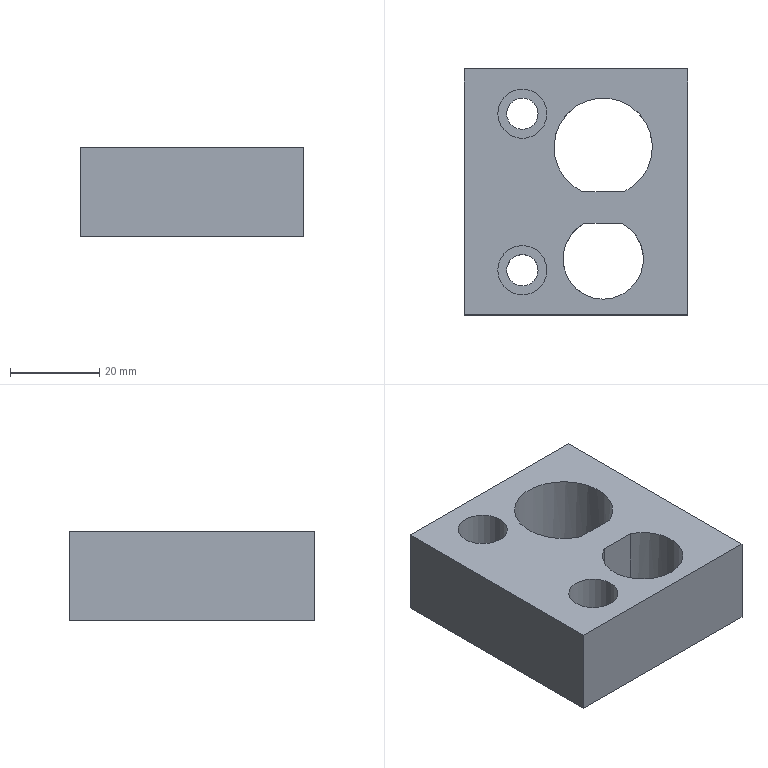Part | STEP file | lll_id706_x_t | 1 solid | 19 faces | box 50 x 55 x 20 mm | volume 39581 mm3 | plane 13 | cylinder 6 | commonest cylinder face diameters 7.009 x2 11.008 x2 18 x1 22 x1
STEP:
#1=CARTESIAN_POINT('',(395.083,115.522,-20.));
#2=VERTEX_POINT('',#1);
#3=CARTESIAN_POINT('',(395.083,107.06,-20.));
#4=VERTEX_POINT('',#3);
#5=CARTESIAN_POINT('',(395.083,100.,-20.));
#6=DIRECTION('',(0.,-1.,0.));
#7=VECTOR('',#6,1.);
#8=LINE('',#5,#7);
#9=EDGE_CURVE('',#2,#4,#8,.T.);
#10=ORIENTED_EDGE('',*,*,#9,.F.);
#11=CARTESIAN_POINT('',(383.917,115.522,-20.));
#12=VERTEX_POINT('',#11);
#13=CARTESIAN_POINT('',(389.5,125.,-20.));
#14=DIRECTION('',(0.,0.,1.));
#15=DIRECTION('',(1.,0.,0.));
#16=AXIS2_PLACEMENT_3D('',#13,#14,#15);
#17=CIRCLE('',#16,11.);
#18=EDGE_CURVE('',#2,#12,#17,.T.);
#19=ORIENTED_EDGE('',*,*,#18,.T.);
#20=CARTESIAN_POINT('',(383.917,107.06,-20.));
#21=VERTEX_POINT('',#20);
#22=CARTESIAN_POINT('',(383.917,100.,-20.));
#23=DIRECTION('',(0.,-1.,0.));
#24=VECTOR('',#23,1.);
#25=LINE('',#22,#24);
#26=EDGE_CURVE('',#12,#21,#25,.T.);
#27=ORIENTED_EDGE('',*,*,#26,.T.);
#28=CARTESIAN_POINT('',(389.5,100.,-20.));
#29=DIRECTION('',(0.,0.,-1.));
#30=DIRECTION('',(-1.,0.,0.));
#31=AXIS2_PLACEMENT_3D('',#28,#29,#30);
#32=CIRCLE('',#31,9.);
#33=EDGE_CURVE('',#4,#21,#32,.T.);
#34=ORIENTED_EDGE('',*,*,#33,.F.);
#35=EDGE_LOOP('',(#10,#19,#27,#34));
#36=FACE_BOUND('',#35,.T.);
#37=CARTESIAN_POINT('',(367.916,97.5,-20.));
#38=VERTEX_POINT('',#37);
#39=CARTESIAN_POINT('',(371.42,97.5,-20.));
#40=DIRECTION('',(0.,0.,-1.));
#41=DIRECTION('',(-1.,0.,0.));
#42=AXIS2_PLACEMENT_3D('',#39,#40,#41);
#43=CIRCLE('',#42,3.505);
#44=EDGE_CURVE('',#38,#38,#43,.T.);
#45=ORIENTED_EDGE('',*,*,#44,.F.);
#46=EDGE_LOOP('',(#45));
#47=FACE_BOUND('',#46,.T.);
#48=CARTESIAN_POINT('',(367.916,132.5,-20.));
#49=VERTEX_POINT('',#48);
#50=CARTESIAN_POINT('',(371.42,132.5,-20.));
#51=DIRECTION('',(0.,0.,-1.));
#52=DIRECTION('',(-1.,0.,0.));
#53=AXIS2_PLACEMENT_3D('',#50,#51,#52);
#54=CIRCLE('',#53,3.505);
#55=EDGE_CURVE('',#49,#49,#54,.T.);
#56=ORIENTED_EDGE('',*,*,#55,.F.);
#57=EDGE_LOOP('',(#56));
#58=FACE_BOUND('',#57,.T.);
#59=CARTESIAN_POINT('',(408.42,87.5,-20.));
#60=VERTEX_POINT('',#59);
#61=CARTESIAN_POINT('',(408.42,142.5,-20.));
#62=VERTEX_POINT('',#61);
#63=CARTESIAN_POINT('',(408.42,111.868,-20.));
#64=DIRECTION('',(0.,1.,0.));
#65=VECTOR('',#64,1.);
#66=LINE('',#63,#65);
#67=EDGE_CURVE('',#60,#62,#66,.T.);
#68=ORIENTED_EDGE('',*,*,#67,.F.);
#69=CARTESIAN_POINT('',(358.42,87.5,-20.));
#70=VERTEX_POINT('',#69);
#71=CARTESIAN_POINT('',(389.5,87.5,-20.));
#72=DIRECTION('',(1.,0.,0.));
#73=VECTOR('',#72,1.);
#74=LINE('',#71,#73);
#75=EDGE_CURVE('',#70,#60,#74,.T.);
#76=ORIENTED_EDGE('',*,*,#75,.F.);
#77=CARTESIAN_POINT('',(358.42,142.5,-20.));
#78=VERTEX_POINT('',#77);
#79=CARTESIAN_POINT('',(358.42,100.,-20.));
#80=DIRECTION('',(0.,-1.,0.));
#81=VECTOR('',#80,1.);
#82=LINE('',#79,#81);
#83=EDGE_CURVE('',#78,#70,#82,.T.);
#84=ORIENTED_EDGE('',*,*,#83,.F.);
#85=CARTESIAN_POINT('',(389.5,142.5,-20.));
#86=DIRECTION('',(-1.,0.,0.));
#87=VECTOR('',#86,1.);
#88=LINE('',#85,#87);
#89=EDGE_CURVE('',#62,#78,#88,.T.);
#90=ORIENTED_EDGE('',*,*,#89,.F.);
#91=EDGE_LOOP('',(#68,#76,#84,#90));
#92=FACE_BOUND('',#91,.T.);
#93=CARTESIAN_POINT('',(389.5,100.,-20.));
#94=DIRECTION('',(0.,0.,-1.));
#95=DIRECTION('',(-1.,0.,0.));
#96=AXIS2_PLACEMENT_3D('',#93,#94,#95);
#97=PLANE('',#96);
#98=ADVANCED_FACE('',(#36,#47,#58,#92),#97,.T.);
#99=CARTESIAN_POINT('',(376.924,97.5,0.));
#100=VERTEX_POINT('',#99);
#101=CARTESIAN_POINT('',(371.42,97.5,0.));
#102=DIRECTION('',(0.,0.,1.));
#103=DIRECTION('',(1.,0.,0.));
#104=AXIS2_PLACEMENT_3D('',#101,#102,#103);
#105=CIRCLE('',#104,5.504);
#106=EDGE_CURVE('',#100,#100,#105,.T.);
#107=ORIENTED_EDGE('',*,*,#106,.F.);
#108=EDGE_LOOP('',(#107));
#109=FACE_BOUND('',#108,.T.);
#110=CARTESIAN_POINT('',(376.924,132.5,0.));
#111=VERTEX_POINT('',#110);
#112=CARTESIAN_POINT('',(371.42,132.5,0.));
#113=DIRECTION('',(0.,0.,1.));
#114=DIRECTION('',(1.,0.,0.));
#115=AXIS2_PLACEMENT_3D('',#112,#113,#114);
#116=CIRCLE('',#115,5.504);
#117=EDGE_CURVE('',#111,#111,#116,.T.);
#118=ORIENTED_EDGE('',*,*,#117,.F.);
#119=EDGE_LOOP('',(#118));
#120=FACE_BOUND('',#119,.T.);
#121=CARTESIAN_POINT('',(408.42,87.5,0.));
#122=VERTEX_POINT('',#121);
#123=CARTESIAN_POINT('',(358.42,87.5,0.));
#124=VERTEX_POINT('',#123);
#125=CARTESIAN_POINT('',(389.5,87.5,0.));
#126=DIRECTION('',(-1.,0.,0.));
#127=VECTOR('',#126,1.);
#128=LINE('',#125,#127);
#129=EDGE_CURVE('',#122,#124,#128,.T.);
#130=ORIENTED_EDGE('',*,*,#129,.F.);
#131=CARTESIAN_POINT('',(408.42,142.5,0.));
#132=VERTEX_POINT('',#131);
#133=CARTESIAN_POINT('',(408.42,111.868,0.));
#134=DIRECTION('',(0.,-1.,0.));
#135=VECTOR('',#134,1.);
#136=LINE('',#133,#135);
#137=EDGE_CURVE('',#132,#122,#136,.T.);
#138=ORIENTED_EDGE('',*,*,#137,.F.);
#139=CARTESIAN_POINT('',(358.42,142.5,0.));
#140=VERTEX_POINT('',#139);
#141=CARTESIAN_POINT('',(389.5,142.5,0.));
#142=DIRECTION('',(1.,0.,0.));
#143=VECTOR('',#142,1.);
#144=LINE('',#141,#143);
#145=EDGE_CURVE('',#140,#132,#144,.T.);
#146=ORIENTED_EDGE('',*,*,#145,.F.);
#147=CARTESIAN_POINT('',(358.42,100.,0.));
#148=DIRECTION('',(0.,1.,0.));
#149=VECTOR('',#148,1.);
#150=LINE('',#147,#149);
#151=EDGE_CURVE('',#124,#140,#150,.T.);
#152=ORIENTED_EDGE('',*,*,#151,.F.);
#153=EDGE_LOOP('',(#130,#138,#146,#152));
#154=FACE_BOUND('',#153,.T.);
#155=CARTESIAN_POINT('',(385.377,108.,0.));
#156=VERTEX_POINT('',#155);
#157=CARTESIAN_POINT('',(393.623,108.,0.));
#158=VERTEX_POINT('',#157);
#159=CARTESIAN_POINT('',(389.5,100.,0.));
#160=DIRECTION('',(0.,0.,1.));
#161=DIRECTION('',(1.,0.,0.));
#162=AXIS2_PLACEMENT_3D('',#159,#160,#161);
#163=CIRCLE('',#162,9.);
#164=EDGE_CURVE('',#156,#158,#163,.T.);
#165=ORIENTED_EDGE('',*,*,#164,.F.);
#166=CARTESIAN_POINT('',(389.5,108.,0.));
#167=DIRECTION('',(1.,0.,0.));
#168=VECTOR('',#167,1.);
#169=LINE('',#166,#168);
#170=EDGE_CURVE('',#156,#158,#169,.T.);
#171=ORIENTED_EDGE('',*,*,#170,.T.);
#172=EDGE_LOOP('',(#165,#171));
#173=FACE_BOUND('',#172,.T.);
#174=CARTESIAN_POINT('',(384.917,115.,0.));
#175=VERTEX_POINT('',#174);
#176=CARTESIAN_POINT('',(394.083,115.,0.));
#177=VERTEX_POINT('',#176);
#178=CARTESIAN_POINT('',(389.5,115.,0.));
#179=DIRECTION('',(1.,0.,0.));
#180=VECTOR('',#179,1.);
#181=LINE('',#178,#180);
#182=EDGE_CURVE('',#175,#177,#181,.T.);
#183=ORIENTED_EDGE('',*,*,#182,.F.);
#184=CARTESIAN_POINT('',(389.5,125.,0.));
#185=DIRECTION('',(0.,0.,-1.));
#186=DIRECTION('',(1.,0.,0.));
#187=AXIS2_PLACEMENT_3D('',#184,#185,#186);
#188=CIRCLE('',#187,11.);
#189=EDGE_CURVE('',#175,#177,#188,.T.);
#190=ORIENTED_EDGE('',*,*,#189,.T.);
#191=EDGE_LOOP('',(#183,#190));
#192=FACE_BOUND('',#191,.T.);
#193=CARTESIAN_POINT('',(389.5,100.,0.));
#194=DIRECTION('',(0.,0.,1.));
#195=DIRECTION('',(1.,0.,0.));
#196=AXIS2_PLACEMENT_3D('',#193,#194,#195);
#197=PLANE('',#196);
#198=ADVANCED_FACE('',(#109,#120,#154,#173,#192),#197,.T.);
#199=CARTESIAN_POINT('',(358.42,87.5,-20.));
#200=DIRECTION('',(0.,0.,1.));
#201=VECTOR('',#200,1.);
#202=LINE('',#199,#201);
#203=EDGE_CURVE('',#70,#124,#202,.T.);
#204=ORIENTED_EDGE('',*,*,#203,.T.);
#205=ORIENTED_EDGE('',*,*,#151,.T.);
#206=CARTESIAN_POINT('',(358.42,142.5,-20.));
#207=DIRECTION('',(0.,0.,1.));
#208=VECTOR('',#207,1.);
#209=LINE('',#206,#208);
#210=EDGE_CURVE('',#78,#140,#209,.T.);
#211=ORIENTED_EDGE('',*,*,#210,.F.);
#212=ORIENTED_EDGE('',*,*,#83,.T.);
#213=EDGE_LOOP('',(#204,#205,#211,#212));
#214=FACE_OUTER_BOUND('',#213,.T.);
#215=CARTESIAN_POINT('',(358.42,100.,-20.));
#216=DIRECTION('',(-1.,0.,0.));
#217=DIRECTION('',(0.,0.,1.));
#218=AXIS2_PLACEMENT_3D('',#215,#216,#217);
#219=PLANE('',#218);
#220=ADVANCED_FACE('',(#214),#219,.T.);
#221=CARTESIAN_POINT('',(408.42,87.5,-20.));
#222=DIRECTION('',(0.,0.,1.));
#223=VECTOR('',#222,1.);
#224=LINE('',#221,#223);
#225=EDGE_CURVE('',#60,#122,#224,.T.);
#226=ORIENTED_EDGE('',*,*,#225,.T.);
#227=ORIENTED_EDGE('',*,*,#129,.T.);
#228=ORIENTED_EDGE('',*,*,#203,.F.);
#229=ORIENTED_EDGE('',*,*,#75,.T.);
#230=EDGE_LOOP('',(#226,#227,#228,#229));
#231=FACE_OUTER_BOUND('',#230,.T.);
#232=CARTESIAN_POINT('',(389.5,87.5,-20.));
#233=DIRECTION('',(0.,-1.,0.));
#234=DIRECTION('',(0.,0.,-1.));
#235=AXIS2_PLACEMENT_3D('',#232,#233,#234);
#236=PLANE('',#235);
#237=ADVANCED_FACE('',(#231),#236,.T.);
#238=ORIENTED_EDGE('',*,*,#67,.T.);
#239=CARTESIAN_POINT('',(408.42,142.5,-16.5));
#240=DIRECTION('',(0.,0.,1.));
#241=VECTOR('',#240,1.);
#242=LINE('',#239,#241);
#243=EDGE_CURVE('',#62,#132,#242,.T.);
#244=ORIENTED_EDGE('',*,*,#243,.T.);
#245=ORIENTED_EDGE('',*,*,#137,.T.);
#246=ORIENTED_EDGE('',*,*,#225,.F.);
#247=EDGE_LOOP('',(#238,#244,#245,#246));
#248=FACE_OUTER_BOUND('',#247,.T.);
#249=CARTESIAN_POINT('',(408.42,111.868,-16.5));
#250=DIRECTION('',(1.,0.,0.));
#251=DIRECTION('',(0.,0.,-1.));
#252=AXIS2_PLACEMENT_3D('',#249,#250,#251);
#253=PLANE('',#252);
#254=ADVANCED_FACE('',(#248),#253,.T.);
#255=CARTESIAN_POINT('',(395.083,107.06,-15.));
#256=VERTEX_POINT('',#255);
#257=CARTESIAN_POINT('',(393.623,108.,-15.));
#258=VERTEX_POINT('',#257);
#259=CARTESIAN_POINT('',(389.5,100.,-15.));
#260=DIRECTION('',(0.,0.,1.));
#261=DIRECTION('',(-1.,0.,0.));
#262=AXIS2_PLACEMENT_3D('',#259,#260,#261);
#263=CIRCLE('',#262,9.);
#264=EDGE_CURVE('',#256,#258,#263,.T.);
#265=ORIENTED_EDGE('',*,*,#264,.F.);
#266=CARTESIAN_POINT('',(395.083,107.06,-15.));
#267=DIRECTION('',(0.,0.,-1.));
#268=VECTOR('',#267,1.);
#269=LINE('',#266,#268);
#270=EDGE_CURVE('',#256,#4,#269,.T.);
#271=ORIENTED_EDGE('',*,*,#270,.T.);
#272=ORIENTED_EDGE('',*,*,#33,.T.);
#273=CARTESIAN_POINT('',(383.917,107.06,-15.));
#274=VERTEX_POINT('',#273);
#275=CARTESIAN_POINT('',(383.917,107.06,0.));
#276=DIRECTION('',(0.,0.,-1.));
#277=VECTOR('',#276,1.);
#278=LINE('',#275,#277);
#279=EDGE_CURVE('',#274,#21,#278,.T.);
#280=ORIENTED_EDGE('',*,*,#279,.F.);
#281=CARTESIAN_POINT('',(385.377,108.,-15.));
#282=VERTEX_POINT('',#281);
#283=CARTESIAN_POINT('',(389.5,100.,-15.));
#284=DIRECTION('',(0.,0.,1.));
#285=DIRECTION('',(-1.,0.,0.));
#286=AXIS2_PLACEMENT_3D('',#283,#284,#285);
#287=CIRCLE('',#286,9.);
#288=EDGE_CURVE('',#282,#274,#287,.T.);
#289=ORIENTED_EDGE('',*,*,#288,.F.);
#290=CARTESIAN_POINT('',(385.377,108.,0.));
#291=DIRECTION('',(0.,0.,-1.));
#292=VECTOR('',#291,1.);
#293=LINE('',#290,#292);
#294=EDGE_CURVE('',#156,#282,#293,.T.);
#295=ORIENTED_EDGE('',*,*,#294,.F.);
#296=ORIENTED_EDGE('',*,*,#164,.T.);
#297=CARTESIAN_POINT('',(393.623,108.,0.));
#298=DIRECTION('',(0.,0.,1.));
#299=VECTOR('',#298,1.);
#300=LINE('',#297,#299);
#301=EDGE_CURVE('',#258,#158,#300,.T.);
#302=ORIENTED_EDGE('',*,*,#301,.F.);
#303=EDGE_LOOP('',(#265,#271,#272,#280,#289,#295,#296,#302));
#304=FACE_OUTER_BOUND('',#303,.T.);
#305=CARTESIAN_POINT('',(389.5,100.,0.));
#306=DIRECTION('',(0.,0.,-1.));
#307=DIRECTION('',(1.,0.,0.));
#308=AXIS2_PLACEMENT_3D('',#305,#306,#307);
#309=CYLINDRICAL_SURFACE('',#308,9.);
#310=ADVANCED_FACE('',(#304),#309,.F.);
#311=CARTESIAN_POINT('',(393.623,108.,-15.));
#312=DIRECTION('',(-1.,0.,0.));
#313=VECTOR('',#312,1.);
#314=LINE('',#311,#313);
#315=EDGE_CURVE('',#258,#282,#314,.T.);
#316=ORIENTED_EDGE('',*,*,#315,.F.);
#317=ORIENTED_EDGE('',*,*,#301,.T.);
#318=ORIENTED_EDGE('',*,*,#170,.F.);
#319=ORIENTED_EDGE('',*,*,#294,.T.);
#320=EDGE_LOOP('',(#316,#317,#318,#319));
#321=FACE_OUTER_BOUND('',#320,.T.);
#322=CARTESIAN_POINT('',(389.5,108.,-10.));
#323=DIRECTION('',(0.,-1.,0.));
#324=DIRECTION('',(0.,0.,1.));
#325=AXIS2_PLACEMENT_3D('',#322,#323,#324);
#326=PLANE('',#325);
#327=ADVANCED_FACE('',(#321),#326,.T.);
#328=ORIENTED_EDGE('',*,*,#210,.T.);
#329=ORIENTED_EDGE('',*,*,#145,.T.);
#330=ORIENTED_EDGE('',*,*,#243,.F.);
#331=ORIENTED_EDGE('',*,*,#89,.T.);
#332=EDGE_LOOP('',(#328,#329,#330,#331));
#333=FACE_OUTER_BOUND('',#332,.T.);
#334=CARTESIAN_POINT('',(389.5,142.5,-20.));
#335=DIRECTION('',(0.,1.,0.));
#336=DIRECTION('',(0.,0.,1.));
#337=AXIS2_PLACEMENT_3D('',#334,#335,#336);
#338=PLANE('',#337);
#339=ADVANCED_FACE('',(#333),#338,.T.);
#340=ORIENTED_EDGE('',*,*,#18,.F.);
#341=CARTESIAN_POINT('',(395.083,115.522,-15.));
#342=VERTEX_POINT('',#341);
#343=CARTESIAN_POINT('',(395.083,115.522,0.));
#344=DIRECTION('',(0.,0.,1.));
#345=VECTOR('',#344,1.);
#346=LINE('',#343,#345);
#347=EDGE_CURVE('',#2,#342,#346,.T.);
#348=ORIENTED_EDGE('',*,*,#347,.T.);
#349=CARTESIAN_POINT('',(394.083,115.,-15.));
#350=VERTEX_POINT('',#349);
#351=CARTESIAN_POINT('',(389.5,125.,-15.));
#352=DIRECTION('',(0.,0.,1.));
#353=DIRECTION('',(1.,0.,0.));
#354=AXIS2_PLACEMENT_3D('',#351,#352,#353);
#355=CIRCLE('',#354,11.);
#356=EDGE_CURVE('',#350,#342,#355,.T.);
#357=ORIENTED_EDGE('',*,*,#356,.F.);
#358=CARTESIAN_POINT('',(394.083,115.,0.));
#359=DIRECTION('',(0.,0.,1.));
#360=VECTOR('',#359,1.);
#361=LINE('',#358,#360);
#362=EDGE_CURVE('',#350,#177,#361,.T.);
#363=ORIENTED_EDGE('',*,*,#362,.T.);
#364=ORIENTED_EDGE('',*,*,#189,.F.);
#365=CARTESIAN_POINT('',(384.917,115.,-15.));
#366=VERTEX_POINT('',#365);
#367=CARTESIAN_POINT('',(384.917,115.,0.));
#368=DIRECTION('',(0.,0.,-1.));
#369=VECTOR('',#368,1.);
#370=LINE('',#367,#369);
#371=EDGE_CURVE('',#175,#366,#370,.T.);
#372=ORIENTED_EDGE('',*,*,#371,.T.);
#373=CARTESIAN_POINT('',(383.917,115.522,-15.));
#374=VERTEX_POINT('',#373);
#375=CARTESIAN_POINT('',(389.5,125.,-15.));
#376=DIRECTION('',(0.,0.,1.));
#377=DIRECTION('',(1.,0.,0.));
#378=AXIS2_PLACEMENT_3D('',#375,#376,#377);
#379=CIRCLE('',#378,11.);
#380=EDGE_CURVE('',#374,#366,#379,.T.);
#381=ORIENTED_EDGE('',*,*,#380,.F.);
#382=CARTESIAN_POINT('',(383.917,115.522,0.));
#383=DIRECTION('',(0.,0.,1.));
#384=VECTOR('',#383,1.);
#385=LINE('',#382,#384);
#386=EDGE_CURVE('',#12,#374,#385,.T.);
#387=ORIENTED_EDGE('',*,*,#386,.F.);
#388=EDGE_LOOP('',(#340,#348,#357,#363,#364,#372,#381,#387));
#389=FACE_OUTER_BOUND('',#388,.T.);
#390=CARTESIAN_POINT('',(389.5,125.,0.));
#391=DIRECTION('',(0.,0.,-1.));
#392=DIRECTION('',(-1.,0.,0.));
#393=AXIS2_PLACEMENT_3D('',#390,#391,#392);
#394=CYLINDRICAL_SURFACE('',#393,11.);
#395=ADVANCED_FACE('',(#389),#394,.F.);
#396=CARTESIAN_POINT('',(389.5,115.,-15.));
#397=DIRECTION('',(1.,0.,0.));
#398=VECTOR('',#397,1.);
#399=LINE('',#396,#398);
#400=EDGE_CURVE('',#366,#350,#399,.T.);
#401=ORIENTED_EDGE('',*,*,#400,.F.);
#402=ORIENTED_EDGE('',*,*,#371,.F.);
#403=ORIENTED_EDGE('',*,*,#182,.T.);
#404=ORIENTED_EDGE('',*,*,#362,.F.);
#405=EDGE_LOOP('',(#401,#402,#403,#404));
#406=FACE_OUTER_BOUND('',#405,.T.);
#407=CARTESIAN_POINT('',(389.5,115.,-10.));
#408=DIRECTION('',(0.,1.,0.));
#409=DIRECTION('',(0.,0.,1.));
#410=AXIS2_PLACEMENT_3D('',#407,#408,#409);
#411=PLANE('',#410);
#412=ADVANCED_FACE('',(#406),#411,.T.);
#413=ORIENTED_EDGE('',*,*,#400,.T.);
#414=ORIENTED_EDGE('',*,*,#356,.T.);
#415=CARTESIAN_POINT('',(395.083,115.,-15.));
#416=DIRECTION('',(0.,-1.,0.));
#417=VECTOR('',#416,1.);
#418=LINE('',#415,#417);
#419=EDGE_CURVE('',#342,#256,#418,.T.);
#420=ORIENTED_EDGE('',*,*,#419,.T.);
#421=ORIENTED_EDGE('',*,*,#264,.T.);
#422=ORIENTED_EDGE('',*,*,#315,.T.);
#423=ORIENTED_EDGE('',*,*,#288,.T.);
#424=CARTESIAN_POINT('',(383.917,115.,-15.));
#425=DIRECTION('',(0.,-1.,0.));
#426=VECTOR('',#425,1.);
#427=LINE('',#424,#426);
#428=EDGE_CURVE('',#374,#274,#427,.T.);
#429=ORIENTED_EDGE('',*,*,#428,.F.);
#430=ORIENTED_EDGE('',*,*,#380,.T.);
#431=EDGE_LOOP('',(#413,#414,#420,#421,#422,#423,#429,#430));
#432=FACE_OUTER_BOUND('',#431,.T.);
#433=CARTESIAN_POINT('',(389.5,125.,-15.));
#434=DIRECTION('',(0.,0.,1.));
#435=DIRECTION('',(1.,0.,0.));
#436=AXIS2_PLACEMENT_3D('',#433,#434,#435);
#437=PLANE('',#436);
#438=ADVANCED_FACE('',(#432),#437,.F.);
#439=ORIENTED_EDGE('',*,*,#55,.T.);
#440=EDGE_LOOP('',(#439));
#441=FACE_BOUND('',#440,.T.);
#442=CARTESIAN_POINT('',(367.916,132.5,-9.));
#443=VERTEX_POINT('',#442);
#444=CARTESIAN_POINT('',(371.42,132.5,-9.));
#445=DIRECTION('',(0.,0.,-1.));
#446=DIRECTION('',(-1.,0.,0.));
#447=AXIS2_PLACEMENT_3D('',#444,#445,#446);
#448=CIRCLE('',#447,3.505);
#449=EDGE_CURVE('',#443,#443,#448,.T.);
#450=ORIENTED_EDGE('',*,*,#449,.F.);
#451=EDGE_LOOP('',(#450));
#452=FACE_BOUND('',#451,.T.);
#453=CARTESIAN_POINT('',(371.42,132.5,2.));
#454=DIRECTION('',(0.,0.,-1.));
#455=DIRECTION('',(1.,0.,0.));
#456=AXIS2_PLACEMENT_3D('',#453,#454,#455);
#457=CYLINDRICAL_SURFACE('',#456,3.505);
#458=ADVANCED_FACE('',(#441,#452),#457,.F.);
#459=ORIENTED_EDGE('',*,*,#449,.T.);
#460=EDGE_LOOP('',(#459));
#461=FACE_BOUND('',#460,.T.);
#462=CARTESIAN_POINT('',(365.916,132.5,-9.));
#463=VERTEX_POINT('',#462);
#464=CARTESIAN_POINT('',(371.42,132.5,-9.));
#465=DIRECTION('',(0.,0.,-1.));
#466=DIRECTION('',(-1.,0.,0.));
#467=AXIS2_PLACEMENT_3D('',#464,#465,#466);
#468=CIRCLE('',#467,5.504);
#469=EDGE_CURVE('',#463,#463,#468,.T.);
#470=ORIENTED_EDGE('',*,*,#469,.F.);
#471=EDGE_LOOP('',(#470));
#472=FACE_BOUND('',#471,.T.);
#473=CARTESIAN_POINT('',(371.42,132.5,-9.));
#474=DIRECTION('',(0.,0.,-1.));
#475=DIRECTION('',(1.,0.,0.));
#476=AXIS2_PLACEMENT_3D('',#473,#474,#475);
#477=PLANE('',#476);
#478=ADVANCED_FACE('',(#461,#472),#477,.F.);
#479=ORIENTED_EDGE('',*,*,#117,.T.);
#480=EDGE_LOOP('',(#479));
#481=FACE_BOUND('',#480,.T.);
#482=ORIENTED_EDGE('',*,*,#469,.T.);
#483=EDGE_LOOP('',(#482));
#484=FACE_BOUND('',#483,.T.);
#485=CARTESIAN_POINT('',(371.42,132.5,0.000025));
#486=DIRECTION('',(0.,0.,-1.));
#487=DIRECTION('',(1.,0.,0.));
#488=AXIS2_PLACEMENT_3D('',#485,#486,#487);
#489=CYLINDRICAL_SURFACE('',#488,5.504);
#490=ADVANCED_FACE('',(#481,#484),#489,.F.);
#491=ORIENTED_EDGE('',*,*,#44,.T.);
#492=EDGE_LOOP('',(#491));
#493=FACE_BOUND('',#492,.T.);
#494=CARTESIAN_POINT('',(367.916,97.5,-9.));
#495=VERTEX_POINT('',#494);
#496=CARTESIAN_POINT('',(371.42,97.5,-9.));
#497=DIRECTION('',(0.,0.,-1.));
#498=DIRECTION('',(-1.,0.,0.));
#499=AXIS2_PLACEMENT_3D('',#496,#497,#498);
#500=CIRCLE('',#499,3.505);
#501=EDGE_CURVE('',#495,#495,#500,.T.);
#502=ORIENTED_EDGE('',*,*,#501,.F.);
#503=EDGE_LOOP('',(#502));
#504=FACE_BOUND('',#503,.T.);
#505=CARTESIAN_POINT('',(371.42,97.5,2.));
#506=DIRECTION('',(0.,0.,-1.));
#507=DIRECTION('',(1.,0.,0.));
#508=AXIS2_PLACEMENT_3D('',#505,#506,#507);
#509=CYLINDRICAL_SURFACE('',#508,3.505);
#510=ADVANCED_FACE('',(#493,#504),#509,.F.);
#511=ORIENTED_EDGE('',*,*,#501,.T.);
#512=EDGE_LOOP('',(#511));
#513=FACE_BOUND('',#512,.T.);
#514=CARTESIAN_POINT('',(365.916,97.5,-9.));
#515=VERTEX_POINT('',#514);
#516=CARTESIAN_POINT('',(371.42,97.5,-9.));
#517=DIRECTION('',(0.,0.,-1.));
#518=DIRECTION('',(-1.,0.,0.));
#519=AXIS2_PLACEMENT_3D('',#516,#517,#518);
#520=CIRCLE('',#519,5.504);
#521=EDGE_CURVE('',#515,#515,#520,.T.);
#522=ORIENTED_EDGE('',*,*,#521,.F.);
#523=EDGE_LOOP('',(#522));
#524=FACE_BOUND('',#523,.T.);
#525=CARTESIAN_POINT('',(371.42,97.5,-9.));
#526=DIRECTION('',(0.,0.,-1.));
#527=DIRECTION('',(1.,0.,0.));
#528=AXIS2_PLACEMENT_3D('',#525,#526,#527);
#529=PLANE('',#528);
#530=ADVANCED_FACE('',(#513,#524),#529,.F.);
#531=ORIENTED_EDGE('',*,*,#106,.T.);
#532=EDGE_LOOP('',(#531));
#533=FACE_BOUND('',#532,.T.);
#534=ORIENTED_EDGE('',*,*,#521,.T.);
#535=EDGE_LOOP('',(#534));
#536=FACE_BOUND('',#535,.T.);
#537=CARTESIAN_POINT('',(371.42,97.5,0.000025));
#538=DIRECTION('',(0.,0.,-1.));
#539=DIRECTION('',(1.,0.,0.));
#540=AXIS2_PLACEMENT_3D('',#537,#538,#539);
#541=CYLINDRICAL_SURFACE('',#540,5.504);
#542=ADVANCED_FACE('',(#533,#536),#541,.F.);
#543=ORIENTED_EDGE('',*,*,#9,.T.);
#544=ORIENTED_EDGE('',*,*,#270,.F.);
#545=ORIENTED_EDGE('',*,*,#419,.F.);
#546=ORIENTED_EDGE('',*,*,#347,.F.);
#547=EDGE_LOOP('',(#543,#544,#545,#546));
#548=FACE_OUTER_BOUND('',#547,.T.);
#549=CARTESIAN_POINT('',(395.083,115.,-33.));
#550=DIRECTION('',(1.,0.,0.));
#551=DIRECTION('',(0.,0.,1.));
#552=AXIS2_PLACEMENT_3D('',#549,#550,#551);
#553=PLANE('',#552);
#554=ADVANCED_FACE('',(#548),#553,.F.);
#555=ORIENTED_EDGE('',*,*,#386,.T.);
#556=ORIENTED_EDGE('',*,*,#428,.T.);
#557=ORIENTED_EDGE('',*,*,#279,.T.);
#558=ORIENTED_EDGE('',*,*,#26,.F.);
#559=EDGE_LOOP('',(#555,#556,#557,#558));
#560=FACE_OUTER_BOUND('',#559,.T.);
#561=CARTESIAN_POINT('',(383.917,115.,-33.));
#562=DIRECTION('',(1.,0.,0.));
#563=DIRECTION('',(0.,0.,1.));
#564=AXIS2_PLACEMENT_3D('',#561,#562,#563);
#565=PLANE('',#564);
#566=ADVANCED_FACE('',(#560),#565,.T.);
#567=CLOSED_SHELL('',(#98,#198,#220,#237,#254,#310,#327,#339,#395,#412,#438,#458,#478,#490,#510,#530,#542,#554,#566));
#568=MANIFOLD_SOLID_BREP('',#567);
#569=(LENGTH_UNIT()NAMED_UNIT(*)SI_UNIT(.MILLI.,.METRE.));
#570=UNCERTAINTY_MEASURE_WITH_UNIT(LENGTH_MEASURE(0.00002),#569,'','');
#571=(NAMED_UNIT(*)PLANE_ANGLE_UNIT()SI_UNIT($,.RADIAN.));
#572=PLANE_ANGLE_MEASURE_WITH_UNIT(PLANE_ANGLE_MEASURE(0.01745),#571);
#573=DIMENSIONAL_EXPONENTS(0.,0.,0.,0.,0.,0.,0.);
#574=(CONVERSION_BASED_UNIT('DEGREE',#572)NAMED_UNIT(#573)PLANE_ANGLE_UNIT());
#575=(NAMED_UNIT(*)SI_UNIT($,.STERADIAN.)SOLID_ANGLE_UNIT());
#576=(GEOMETRIC_REPRESENTATION_CONTEXT(3)GLOBAL_UNCERTAINTY_ASSIGNED_CONTEXT((#570))GLOBAL_UNIT_ASSIGNED_CONTEXT((#569,#574,#575))REPRESENTATION_CONTEXT('',''));
#577=ADVANCED_BREP_SHAPE_REPRESENTATION('',(#568),#576);